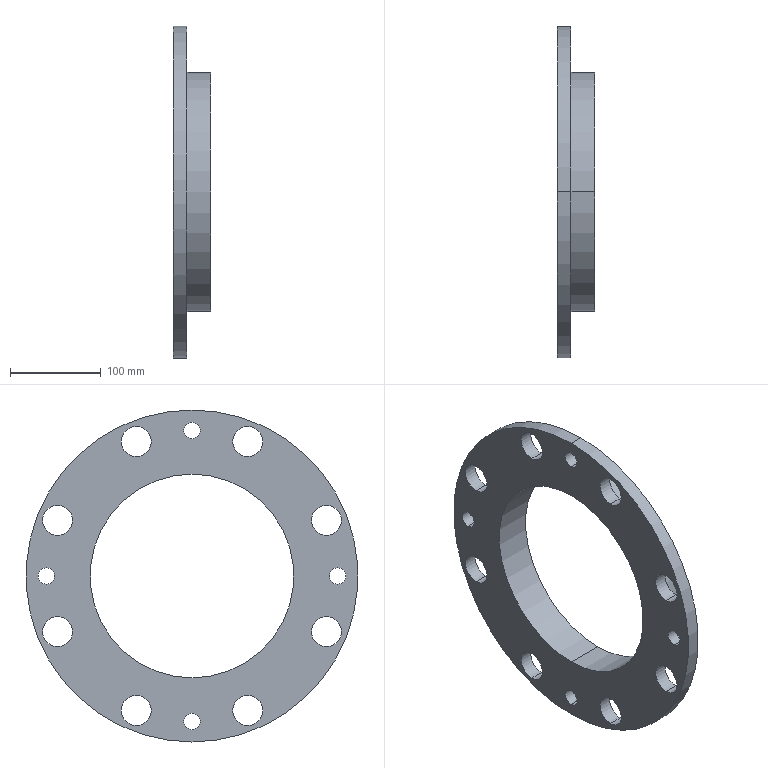Part | SolidWorks | features ICE 2, Revolution 1 | 1 solid | 33 faces | box 41 x 365 x 365 mm | volume 1248338 mm3 | cylinder 30 | plane 3 | commonest cylinder face diameters 33 x16 18 x8 224 x2 263 x2 365 x2
STEP:
#1=CARTESIAN_POINT('',(-4.589,0.,-169.));
#2=VERTEX_POINT('',#1);
#3=CARTESIAN_POINT('',(-4.589,0.,-151.));
#4=VERTEX_POINT('',#3);
#5=CARTESIAN_POINT('',(-4.589,0.,-160.));
#6=DIRECTION('',(-1.,0.,0.));
#7=DIRECTION('',(0.,0.,1.));
#8=AXIS2_PLACEMENT_3D('',#5,#6,#7);
#9=CIRCLE('',#8,9.);
#10=EDGE_CURVE('',#2,#4,#9,.T.);
#11=ORIENTED_EDGE('',*,*,#10,.F.);
#12=CARTESIAN_POINT('',(-19.589,0.,-169.));
#13=VERTEX_POINT('',#12);
#14=CARTESIAN_POINT('',(0.411,0.,-169.));
#15=DIRECTION('',(-1.,0.,0.));
#16=VECTOR('',#15,1000.);
#17=LINE('',#14,#16);
#18=EDGE_CURVE('',#2,#13,#17,.T.);
#19=ORIENTED_EDGE('',*,*,#18,.T.);
#20=CARTESIAN_POINT('',(-19.589,0.,-151.));
#21=VERTEX_POINT('',#20);
#22=CARTESIAN_POINT('',(-19.589,0.,-160.));
#23=DIRECTION('',(-1.,0.,0.));
#24=DIRECTION('',(0.,0.,1.));
#25=AXIS2_PLACEMENT_3D('',#22,#23,#24);
#26=CIRCLE('',#25,9.);
#27=EDGE_CURVE('',#13,#21,#26,.T.);
#28=ORIENTED_EDGE('',*,*,#27,.T.);
#29=CARTESIAN_POINT('',(0.411,0.,-151.));
#30=DIRECTION('',(-1.,0.,0.));
#31=VECTOR('',#30,1000.);
#32=LINE('',#29,#31);
#33=EDGE_CURVE('',#4,#21,#32,.T.);
#34=ORIENTED_EDGE('',*,*,#33,.F.);
#35=EDGE_LOOP('',(#11,#19,#28,#34));
#36=FACE_OUTER_BOUND('',#35,.T.);
#37=CARTESIAN_POINT('',(0.411,0.,-160.));
#38=DIRECTION('',(-1.,0.,0.));
#39=DIRECTION('',(0.,0.,1.));
#40=AXIS2_PLACEMENT_3D('',#37,#38,#39);
#41=CYLINDRICAL_SURFACE('',#40,9.);
#42=ADVANCED_FACE('',(#36),#41,.F.);
#43=CARTESIAN_POINT('',(-4.589,-160.,-9.));
#44=VERTEX_POINT('',#43);
#45=CARTESIAN_POINT('',(-4.589,-160.,9.));
#46=VERTEX_POINT('',#45);
#47=CARTESIAN_POINT('',(-4.589,-160.,0.));
#48=DIRECTION('',(-1.,0.,0.));
#49=DIRECTION('',(0.,0.,1.));
#50=AXIS2_PLACEMENT_3D('',#47,#48,#49);
#51=CIRCLE('',#50,9.);
#52=EDGE_CURVE('',#44,#46,#51,.T.);
#53=ORIENTED_EDGE('',*,*,#52,.F.);
#54=CARTESIAN_POINT('',(-19.589,-160.,-9.));
#55=VERTEX_POINT('',#54);
#56=CARTESIAN_POINT('',(0.411,-160.,-9.));
#57=DIRECTION('',(-1.,0.,0.));
#58=VECTOR('',#57,1000.);
#59=LINE('',#56,#58);
#60=EDGE_CURVE('',#44,#55,#59,.T.);
#61=ORIENTED_EDGE('',*,*,#60,.T.);
#62=CARTESIAN_POINT('',(-19.589,-160.,9.));
#63=VERTEX_POINT('',#62);
#64=CARTESIAN_POINT('',(-19.589,-160.,0.));
#65=DIRECTION('',(-1.,0.,0.));
#66=DIRECTION('',(0.,0.,1.));
#67=AXIS2_PLACEMENT_3D('',#64,#65,#66);
#68=CIRCLE('',#67,9.);
#69=EDGE_CURVE('',#55,#63,#68,.T.);
#70=ORIENTED_EDGE('',*,*,#69,.T.);
#71=CARTESIAN_POINT('',(0.411,-160.,9.));
#72=DIRECTION('',(-1.,0.,0.));
#73=VECTOR('',#72,1000.);
#74=LINE('',#71,#73);
#75=EDGE_CURVE('',#46,#63,#74,.T.);
#76=ORIENTED_EDGE('',*,*,#75,.F.);
#77=EDGE_LOOP('',(#53,#61,#70,#76));
#78=FACE_OUTER_BOUND('',#77,.T.);
#79=CARTESIAN_POINT('',(0.411,-160.,0.));
#80=DIRECTION('',(-1.,0.,0.));
#81=DIRECTION('',(0.,0.,1.));
#82=AXIS2_PLACEMENT_3D('',#79,#80,#81);
#83=CYLINDRICAL_SURFACE('',#82,9.);
#84=ADVANCED_FACE('',(#78),#83,.F.);
#85=CARTESIAN_POINT('',(-4.589,0.,151.));
#86=VERTEX_POINT('',#85);
#87=CARTESIAN_POINT('',(-4.589,0.,169.));
#88=VERTEX_POINT('',#87);
#89=CARTESIAN_POINT('',(-4.589,0.,160.));
#90=DIRECTION('',(-1.,0.,0.));
#91=DIRECTION('',(0.,0.,1.));
#92=AXIS2_PLACEMENT_3D('',#89,#90,#91);
#93=CIRCLE('',#92,9.);
#94=EDGE_CURVE('',#86,#88,#93,.T.);
#95=ORIENTED_EDGE('',*,*,#94,.F.);
#96=CARTESIAN_POINT('',(-19.589,0.,151.));
#97=VERTEX_POINT('',#96);
#98=CARTESIAN_POINT('',(0.411,0.,151.));
#99=DIRECTION('',(-1.,0.,0.));
#100=VECTOR('',#99,1000.);
#101=LINE('',#98,#100);
#102=EDGE_CURVE('',#86,#97,#101,.T.);
#103=ORIENTED_EDGE('',*,*,#102,.T.);
#104=CARTESIAN_POINT('',(-19.589,0.,169.));
#105=VERTEX_POINT('',#104);
#106=CARTESIAN_POINT('',(-19.589,0.,160.));
#107=DIRECTION('',(-1.,0.,0.));
#108=DIRECTION('',(0.,0.,1.));
#109=AXIS2_PLACEMENT_3D('',#106,#107,#108);
#110=CIRCLE('',#109,9.);
#111=EDGE_CURVE('',#97,#105,#110,.T.);
#112=ORIENTED_EDGE('',*,*,#111,.T.);
#113=CARTESIAN_POINT('',(0.411,0.,169.));
#114=DIRECTION('',(-1.,0.,0.));
#115=VECTOR('',#114,1000.);
#116=LINE('',#113,#115);
#117=EDGE_CURVE('',#88,#105,#116,.T.);
#118=ORIENTED_EDGE('',*,*,#117,.F.);
#119=EDGE_LOOP('',(#95,#103,#112,#118));
#120=FACE_OUTER_BOUND('',#119,.T.);
#121=CARTESIAN_POINT('',(0.411,0.,160.));
#122=DIRECTION('',(-1.,0.,0.));
#123=DIRECTION('',(0.,0.,1.));
#124=AXIS2_PLACEMENT_3D('',#121,#122,#123);
#125=CYLINDRICAL_SURFACE('',#124,9.);
#126=ADVANCED_FACE('',(#120),#125,.F.);
#127=CARTESIAN_POINT('',(-4.589,160.,-9.));
#128=VERTEX_POINT('',#127);
#129=CARTESIAN_POINT('',(-4.589,160.,9.));
#130=VERTEX_POINT('',#129);
#131=CARTESIAN_POINT('',(-4.589,160.,0.));
#132=DIRECTION('',(-1.,0.,0.));
#133=DIRECTION('',(0.,0.,1.));
#134=AXIS2_PLACEMENT_3D('',#131,#132,#133);
#135=CIRCLE('',#134,9.);
#136=EDGE_CURVE('',#128,#130,#135,.T.);
#137=ORIENTED_EDGE('',*,*,#136,.F.);
#138=CARTESIAN_POINT('',(-19.589,160.,-9.));
#139=VERTEX_POINT('',#138);
#140=CARTESIAN_POINT('',(0.411,160.,-9.));
#141=DIRECTION('',(-1.,0.,0.));
#142=VECTOR('',#141,1000.);
#143=LINE('',#140,#142);
#144=EDGE_CURVE('',#128,#139,#143,.T.);
#145=ORIENTED_EDGE('',*,*,#144,.T.);
#146=CARTESIAN_POINT('',(-19.589,160.,9.));
#147=VERTEX_POINT('',#146);
#148=CARTESIAN_POINT('',(-19.589,160.,0.));
#149=DIRECTION('',(-1.,0.,0.));
#150=DIRECTION('',(0.,0.,1.));
#151=AXIS2_PLACEMENT_3D('',#148,#149,#150);
#152=CIRCLE('',#151,9.);
#153=EDGE_CURVE('',#139,#147,#152,.T.);
#154=ORIENTED_EDGE('',*,*,#153,.T.);
#155=CARTESIAN_POINT('',(0.411,160.,9.));
#156=DIRECTION('',(-1.,0.,0.));
#157=VECTOR('',#156,1000.);
#158=LINE('',#155,#157);
#159=EDGE_CURVE('',#130,#147,#158,.T.);
#160=ORIENTED_EDGE('',*,*,#159,.F.);
#161=EDGE_LOOP('',(#137,#145,#154,#160));
#162=FACE_OUTER_BOUND('',#161,.T.);
#163=CARTESIAN_POINT('',(0.411,160.,0.));
#164=DIRECTION('',(-1.,0.,0.));
#165=DIRECTION('',(0.,0.,1.));
#166=AXIS2_PLACEMENT_3D('',#163,#164,#165);
#167=CYLINDRICAL_SURFACE('',#166,9.);
#168=ADVANCED_FACE('',(#162),#167,.F.);
#169=CARTESIAN_POINT('',(-4.589,147.821,-77.729));
#170=VERTEX_POINT('',#169);
#171=CARTESIAN_POINT('',(-4.589,147.821,-44.729));
#172=VERTEX_POINT('',#171);
#173=CARTESIAN_POINT('',(-4.589,147.821,-61.229));
#174=DIRECTION('',(-1.,0.,0.));
#175=DIRECTION('',(0.,0.,1.));
#176=AXIS2_PLACEMENT_3D('',#173,#174,#175);
#177=CIRCLE('',#176,16.5);
#178=EDGE_CURVE('',#170,#172,#177,.T.);
#179=ORIENTED_EDGE('',*,*,#178,.F.);
#180=CARTESIAN_POINT('',(-19.589,147.821,-77.729));
#181=VERTEX_POINT('',#180);
#182=CARTESIAN_POINT('',(0.411,147.821,-77.729));
#183=DIRECTION('',(-1.,0.,0.));
#184=VECTOR('',#183,1000.);
#185=LINE('',#182,#184);
#186=EDGE_CURVE('',#170,#181,#185,.T.);
#187=ORIENTED_EDGE('',*,*,#186,.T.);
#188=CARTESIAN_POINT('',(-19.589,147.821,-44.729));
#189=VERTEX_POINT('',#188);
#190=CARTESIAN_POINT('',(-19.589,147.821,-61.229));
#191=DIRECTION('',(-1.,0.,0.));
#192=DIRECTION('',(0.,0.,1.));
#193=AXIS2_PLACEMENT_3D('',#190,#191,#192);
#194=CIRCLE('',#193,16.5);
#195=EDGE_CURVE('',#181,#189,#194,.T.);
#196=ORIENTED_EDGE('',*,*,#195,.T.);
#197=CARTESIAN_POINT('',(0.411,147.821,-44.729));
#198=DIRECTION('',(-1.,0.,0.));
#199=VECTOR('',#198,1000.);
#200=LINE('',#197,#199);
#201=EDGE_CURVE('',#172,#189,#200,.T.);
#202=ORIENTED_EDGE('',*,*,#201,.F.);
#203=EDGE_LOOP('',(#179,#187,#196,#202));
#204=FACE_OUTER_BOUND('',#203,.T.);
#205=CARTESIAN_POINT('',(0.411,147.821,-61.229));
#206=DIRECTION('',(-1.,0.,0.));
#207=DIRECTION('',(0.,0.,1.));
#208=AXIS2_PLACEMENT_3D('',#205,#206,#207);
#209=CYLINDRICAL_SURFACE('',#208,16.5);
#210=ADVANCED_FACE('',(#204),#209,.F.);
#211=CARTESIAN_POINT('',(-4.589,61.229,-164.321));
#212=VERTEX_POINT('',#211);
#213=CARTESIAN_POINT('',(-4.589,61.229,-131.321));
#214=VERTEX_POINT('',#213);
#215=CARTESIAN_POINT('',(-4.589,61.229,-147.821));
#216=DIRECTION('',(-1.,0.,0.));
#217=DIRECTION('',(0.,0.,1.));
#218=AXIS2_PLACEMENT_3D('',#215,#216,#217);
#219=CIRCLE('',#218,16.5);
#220=EDGE_CURVE('',#212,#214,#219,.T.);
#221=ORIENTED_EDGE('',*,*,#220,.F.);
#222=CARTESIAN_POINT('',(-19.589,61.229,-164.321));
#223=VERTEX_POINT('',#222);
#224=CARTESIAN_POINT('',(0.411,61.229,-164.321));
#225=DIRECTION('',(-1.,0.,0.));
#226=VECTOR('',#225,1000.);
#227=LINE('',#224,#226);
#228=EDGE_CURVE('',#212,#223,#227,.T.);
#229=ORIENTED_EDGE('',*,*,#228,.T.);
#230=CARTESIAN_POINT('',(-19.589,61.229,-131.321));
#231=VERTEX_POINT('',#230);
#232=CARTESIAN_POINT('',(-19.589,61.229,-147.821));
#233=DIRECTION('',(-1.,0.,0.));
#234=DIRECTION('',(0.,0.,1.));
#235=AXIS2_PLACEMENT_3D('',#232,#233,#234);
#236=CIRCLE('',#235,16.5);
#237=EDGE_CURVE('',#223,#231,#236,.T.);
#238=ORIENTED_EDGE('',*,*,#237,.T.);
#239=CARTESIAN_POINT('',(0.411,61.229,-131.321));
#240=DIRECTION('',(-1.,0.,0.));
#241=VECTOR('',#240,1000.);
#242=LINE('',#239,#241);
#243=EDGE_CURVE('',#214,#231,#242,.T.);
#244=ORIENTED_EDGE('',*,*,#243,.F.);
#245=EDGE_LOOP('',(#221,#229,#238,#244));
#246=FACE_OUTER_BOUND('',#245,.T.);
#247=CARTESIAN_POINT('',(0.411,61.229,-147.821));
#248=DIRECTION('',(-1.,0.,0.));
#249=DIRECTION('',(0.,0.,1.));
#250=AXIS2_PLACEMENT_3D('',#247,#248,#249);
#251=CYLINDRICAL_SURFACE('',#250,16.5);
#252=ADVANCED_FACE('',(#246),#251,.F.);
#253=CARTESIAN_POINT('',(-4.589,-61.229,-164.321));
#254=VERTEX_POINT('',#253);
#255=CARTESIAN_POINT('',(-4.589,-61.229,-131.321));
#256=VERTEX_POINT('',#255);
#257=CARTESIAN_POINT('',(-4.589,-61.229,-147.821));
#258=DIRECTION('',(-1.,0.,0.));
#259=DIRECTION('',(0.,0.,1.));
#260=AXIS2_PLACEMENT_3D('',#257,#258,#259);
#261=CIRCLE('',#260,16.5);
#262=EDGE_CURVE('',#254,#256,#261,.T.);
#263=ORIENTED_EDGE('',*,*,#262,.F.);
#264=CARTESIAN_POINT('',(-19.589,-61.229,-164.321));
#265=VERTEX_POINT('',#264);
#266=CARTESIAN_POINT('',(0.411,-61.229,-164.321));
#267=DIRECTION('',(-1.,0.,0.));
#268=VECTOR('',#267,1000.);
#269=LINE('',#266,#268);
#270=EDGE_CURVE('',#254,#265,#269,.T.);
#271=ORIENTED_EDGE('',*,*,#270,.T.);
#272=CARTESIAN_POINT('',(-19.589,-61.229,-131.321));
#273=VERTEX_POINT('',#272);
#274=CARTESIAN_POINT('',(-19.589,-61.229,-147.821));
#275=DIRECTION('',(-1.,0.,0.));
#276=DIRECTION('',(0.,0.,1.));
#277=AXIS2_PLACEMENT_3D('',#274,#275,#276);
#278=CIRCLE('',#277,16.5);
#279=EDGE_CURVE('',#265,#273,#278,.T.);
#280=ORIENTED_EDGE('',*,*,#279,.T.);
#281=CARTESIAN_POINT('',(0.411,-61.229,-131.321));
#282=DIRECTION('',(-1.,0.,0.));
#283=VECTOR('',#282,1000.);
#284=LINE('',#281,#283);
#285=EDGE_CURVE('',#256,#273,#284,.T.);
#286=ORIENTED_EDGE('',*,*,#285,.F.);
#287=EDGE_LOOP('',(#263,#271,#280,#286));
#288=FACE_OUTER_BOUND('',#287,.T.);
#289=CARTESIAN_POINT('',(0.411,-61.229,-147.821));
#290=DIRECTION('',(-1.,0.,0.));
#291=DIRECTION('',(0.,0.,1.));
#292=AXIS2_PLACEMENT_3D('',#289,#290,#291);
#293=CYLINDRICAL_SURFACE('',#292,16.5);
#294=ADVANCED_FACE('',(#288),#293,.F.);
#295=CARTESIAN_POINT('',(-4.589,-147.821,-77.729));
#296=VERTEX_POINT('',#295);
#297=CARTESIAN_POINT('',(-4.589,-147.821,-44.729));
#298=VERTEX_POINT('',#297);
#299=CARTESIAN_POINT('',(-4.589,-147.821,-61.229));
#300=DIRECTION('',(-1.,0.,0.));
#301=DIRECTION('',(0.,0.,1.));
#302=AXIS2_PLACEMENT_3D('',#299,#300,#301);
#303=CIRCLE('',#302,16.5);
#304=EDGE_CURVE('',#296,#298,#303,.T.);
#305=ORIENTED_EDGE('',*,*,#304,.F.);
#306=CARTESIAN_POINT('',(-19.589,-147.821,-77.729));
#307=VERTEX_POINT('',#306);
#308=CARTESIAN_POINT('',(0.411,-147.821,-77.729));
#309=DIRECTION('',(-1.,0.,0.));
#310=VECTOR('',#309,1000.);
#311=LINE('',#308,#310);
#312=EDGE_CURVE('',#296,#307,#311,.T.);
#313=ORIENTED_EDGE('',*,*,#312,.T.);
#314=CARTESIAN_POINT('',(-19.589,-147.821,-44.729));
#315=VERTEX_POINT('',#314);
#316=CARTESIAN_POINT('',(-19.589,-147.821,-61.229));
#317=DIRECTION('',(-1.,0.,0.));
#318=DIRECTION('',(0.,0.,1.));
#319=AXIS2_PLACEMENT_3D('',#316,#317,#318);
#320=CIRCLE('',#319,16.5);
#321=EDGE_CURVE('',#307,#315,#320,.T.);
#322=ORIENTED_EDGE('',*,*,#321,.T.);
#323=CARTESIAN_POINT('',(0.411,-147.821,-44.729));
#324=DIRECTION('',(-1.,0.,0.));
#325=VECTOR('',#324,1000.);
#326=LINE('',#323,#325);
#327=EDGE_CURVE('',#298,#315,#326,.T.);
#328=ORIENTED_EDGE('',*,*,#327,.F.);
#329=EDGE_LOOP('',(#305,#313,#322,#328));
#330=FACE_OUTER_BOUND('',#329,.T.);
#331=CARTESIAN_POINT('',(0.411,-147.821,-61.229));
#332=DIRECTION('',(-1.,0.,0.));
#333=DIRECTION('',(0.,0.,1.));
#334=AXIS2_PLACEMENT_3D('',#331,#332,#333);
#335=CYLINDRICAL_SURFACE('',#334,16.5);
#336=ADVANCED_FACE('',(#330),#335,.F.);
#337=CARTESIAN_POINT('',(-4.589,-147.821,44.729));
#338=VERTEX_POINT('',#337);
#339=CARTESIAN_POINT('',(-4.589,-147.821,77.729));
#340=VERTEX_POINT('',#339);
#341=CARTESIAN_POINT('',(-4.589,-147.821,61.229));
#342=DIRECTION('',(-1.,0.,0.));
#343=DIRECTION('',(0.,0.,1.));
#344=AXIS2_PLACEMENT_3D('',#341,#342,#343);
#345=CIRCLE('',#344,16.5);
#346=EDGE_CURVE('',#338,#340,#345,.T.);
#347=ORIENTED_EDGE('',*,*,#346,.F.);
#348=CARTESIAN_POINT('',(-19.589,-147.821,44.729));
#349=VERTEX_POINT('',#348);
#350=CARTESIAN_POINT('',(0.411,-147.821,44.729));
#351=DIRECTION('',(-1.,0.,0.));
#352=VECTOR('',#351,1000.);
#353=LINE('',#350,#352);
#354=EDGE_CURVE('',#338,#349,#353,.T.);
#355=ORIENTED_EDGE('',*,*,#354,.T.);
#356=CARTESIAN_POINT('',(-19.589,-147.821,77.729));
#357=VERTEX_POINT('',#356);
#358=CARTESIAN_POINT('',(-19.589,-147.821,61.229));
#359=DIRECTION('',(-1.,0.,0.));
#360=DIRECTION('',(0.,0.,1.));
#361=AXIS2_PLACEMENT_3D('',#358,#359,#360);
#362=CIRCLE('',#361,16.5);
#363=EDGE_CURVE('',#349,#357,#362,.T.);
#364=ORIENTED_EDGE('',*,*,#363,.T.);
#365=CARTESIAN_POINT('',(0.411,-147.821,77.729));
#366=DIRECTION('',(-1.,0.,0.));
#367=VECTOR('',#366,1000.);
#368=LINE('',#365,#367);
#369=EDGE_CURVE('',#340,#357,#368,.T.);
#370=ORIENTED_EDGE('',*,*,#369,.F.);
#371=EDGE_LOOP('',(#347,#355,#364,#370));
#372=FACE_OUTER_BOUND('',#371,.T.);
#373=CARTESIAN_POINT('',(0.411,-147.821,61.229));
#374=DIRECTION('',(-1.,0.,0.));
#375=DIRECTION('',(0.,0.,1.));
#376=AXIS2_PLACEMENT_3D('',#373,#374,#375);
#377=CYLINDRICAL_SURFACE('',#376,16.5);
#378=ADVANCED_FACE('',(#372),#377,.F.);
#379=CARTESIAN_POINT('',(-4.589,-61.229,131.321));
#380=VERTEX_POINT('',#379);
#381=CARTESIAN_POINT('',(-4.589,-61.229,164.321));
#382=VERTEX_POINT('',#381);
#383=CARTESIAN_POINT('',(-4.589,-61.229,147.821));
#384=DIRECTION('',(-1.,0.,0.));
#385=DIRECTION('',(0.,0.,1.));
#386=AXIS2_PLACEMENT_3D('',#383,#384,#385);
#387=CIRCLE('',#386,16.5);
#388=EDGE_CURVE('',#380,#382,#387,.T.);
#389=ORIENTED_EDGE('',*,*,#388,.F.);
#390=CARTESIAN_POINT('',(-19.589,-61.229,131.321));
#391=VERTEX_POINT('',#390);
#392=CARTESIAN_POINT('',(0.411,-61.229,131.321));
#393=DIRECTION('',(-1.,0.,0.));
#394=VECTOR('',#393,1000.);
#395=LINE('',#392,#394);
#396=EDGE_CURVE('',#380,#391,#395,.T.);
#397=ORIENTED_EDGE('',*,*,#396,.T.);
#398=CARTESIAN_POINT('',(-19.589,-61.229,164.321));
#399=VERTEX_POINT('',#398);
#400=CARTESIAN_POINT('',(-19.589,-61.229,147.821));
#401=DIRECTION('',(-1.,0.,0.));
#402=DIRECTION('',(0.,0.,1.));
#403=AXIS2_PLACEMENT_3D('',#400,#401,#402);
#404=CIRCLE('',#403,16.5);
#405=EDGE_CURVE('',#391,#399,#404,.T.);
#406=ORIENTED_EDGE('',*,*,#405,.T.);
#407=CARTESIAN_POINT('',(0.411,-61.229,164.321));
#408=DIRECTION('',(-1.,0.,0.));
#409=VECTOR('',#408,1000.);
#410=LINE('',#407,#409);
#411=EDGE_CURVE('',#382,#399,#410,.T.);
#412=ORIENTED_EDGE('',*,*,#411,.F.);
#413=EDGE_LOOP('',(#389,#397,#406,#412));
#414=FACE_OUTER_BOUND('',#413,.T.);
#415=CARTESIAN_POINT('',(0.411,-61.229,147.821));
#416=DIRECTION('',(-1.,0.,0.));
#417=DIRECTION('',(0.,0.,1.));
#418=AXIS2_PLACEMENT_3D('',#415,#416,#417);
#419=CYLINDRICAL_SURFACE('',#418,16.5);
#420=ADVANCED_FACE('',(#414),#419,.F.);
#421=CARTESIAN_POINT('',(-4.589,61.229,131.321));
#422=VERTEX_POINT('',#421);
#423=CARTESIAN_POINT('',(-4.589,61.229,164.321));
#424=VERTEX_POINT('',#423);
#425=CARTESIAN_POINT('',(-4.589,61.229,147.821));
#426=DIRECTION('',(-1.,0.,0.));
#427=DIRECTION('',(0.,0.,1.));
#428=AXIS2_PLACEMENT_3D('',#425,#426,#427);
#429=CIRCLE('',#428,16.5);
#430=EDGE_CURVE('',#422,#424,#429,.T.);
#431=ORIENTED_EDGE('',*,*,#430,.F.);
#432=CARTESIAN_POINT('',(-19.589,61.229,131.321));
#433=VERTEX_POINT('',#432);
#434=CARTESIAN_POINT('',(0.411,61.229,131.321));
#435=DIRECTION('',(-1.,0.,0.));
#436=VECTOR('',#435,1000.);
#437=LINE('',#434,#436);
#438=EDGE_CURVE('',#422,#433,#437,.T.);
#439=ORIENTED_EDGE('',*,*,#438,.T.);
#440=CARTESIAN_POINT('',(-19.589,61.229,164.321));
#441=VERTEX_POINT('',#440);
#442=CARTESIAN_POINT('',(-19.589,61.229,147.821));
#443=DIRECTION('',(-1.,0.,0.));
#444=DIRECTION('',(0.,0.,1.));
#445=AXIS2_PLACEMENT_3D('',#442,#443,#444);
#446=CIRCLE('',#445,16.5);
#447=EDGE_CURVE('',#433,#441,#446,.T.);
#448=ORIENTED_EDGE('',*,*,#447,.T.);
#449=CARTESIAN_POINT('',(0.411,61.229,164.321));
#450=DIRECTION('',(-1.,0.,0.));
#451=VECTOR('',#450,1000.);
#452=LINE('',#449,#451);
#453=EDGE_CURVE('',#424,#441,#452,.T.);
#454=ORIENTED_EDGE('',*,*,#453,.F.);
#455=EDGE_LOOP('',(#431,#439,#448,#454));
#456=FACE_OUTER_BOUND('',#455,.T.);
#457=CARTESIAN_POINT('',(0.411,61.229,147.821));
#458=DIRECTION('',(-1.,0.,0.));
#459=DIRECTION('',(0.,0.,1.));
#460=AXIS2_PLACEMENT_3D('',#457,#458,#459);
#461=CYLINDRICAL_SURFACE('',#460,16.5);
#462=ADVANCED_FACE('',(#456),#461,.F.);
#463=CARTESIAN_POINT('',(-4.589,147.821,44.729));
#464=VERTEX_POINT('',#463);
#465=CARTESIAN_POINT('',(-4.589,147.821,77.729));
#466=VERTEX_POINT('',#465);
#467=CARTESIAN_POINT('',(-4.589,147.821,61.229));
#468=DIRECTION('',(-1.,0.,0.));
#469=DIRECTION('',(0.,0.,1.));
#470=AXIS2_PLACEMENT_3D('',#467,#468,#469);
#471=CIRCLE('',#470,16.5);
#472=EDGE_CURVE('',#464,#466,#471,.T.);
#473=ORIENTED_EDGE('',*,*,#472,.F.);
#474=CARTESIAN_POINT('',(-19.589,147.821,44.729));
#475=VERTEX_POINT('',#474);
#476=CARTESIAN_POINT('',(0.411,147.821,44.729));
#477=DIRECTION('',(-1.,0.,0.));
#478=VECTOR('',#477,1000.);
#479=LINE('',#476,#478);
#480=EDGE_CURVE('',#464,#475,#479,.T.);
#481=ORIENTED_EDGE('',*,*,#480,.T.);
#482=CARTESIAN_POINT('',(-19.589,147.821,77.729));
#483=VERTEX_POINT('',#482);
#484=CARTESIAN_POINT('',(-19.589,147.821,61.229));
#485=DIRECTION('',(-1.,0.,0.));
#486=DIRECTION('',(0.,0.,1.));
#487=AXIS2_PLACEMENT_3D('',#484,#485,#486);
#488=CIRCLE('',#487,16.5);
#489=EDGE_CURVE('',#475,#483,#488,.T.);
#490=ORIENTED_EDGE('',*,*,#489,.T.);
#491=CARTESIAN_POINT('',(0.411,147.821,77.729));
#492=DIRECTION('',(-1.,0.,0.));
#493=VECTOR('',#492,1000.);
#494=LINE('',#491,#493);
#495=EDGE_CURVE('',#466,#483,#494,.T.);
#496=ORIENTED_EDGE('',*,*,#495,.F.);
#497=EDGE_LOOP('',(#473,#481,#490,#496));
#498=FACE_OUTER_BOUND('',#497,.T.);
#499=CARTESIAN_POINT('',(0.411,147.821,61.229));
#500=DIRECTION('',(-1.,0.,0.));
#501=DIRECTION('',(0.,0.,1.));
#502=AXIS2_PLACEMENT_3D('',#499,#500,#501);
#503=CYLINDRICAL_SURFACE('',#502,16.5);
#504=ADVANCED_FACE('',(#498),#503,.F.);
#505=CARTESIAN_POINT('',(21.411,0.,131.5));
#506=VERTEX_POINT('',#505);
#507=CARTESIAN_POINT('',(21.411,0.,-131.5));
#508=VERTEX_POINT('',#507);
#509=CARTESIAN_POINT('',(21.411,0.,0.));
#510=DIRECTION('',(-1.,0.,0.));
#511=DIRECTION('',(0.,0.,1.));
#512=AXIS2_PLACEMENT_3D('',#509,#510,#511);
#513=CIRCLE('',#512,131.5);
#514=EDGE_CURVE('',#506,#508,#513,.T.);
#515=ORIENTED_EDGE('',*,*,#514,.T.);
#516=CARTESIAN_POINT('',(-4.589,0.,-131.5));
#517=VERTEX_POINT('',#516);
#518=CARTESIAN_POINT('',(-91.426,0.,-131.5));
#519=DIRECTION('',(-1.,0.,0.));
#520=VECTOR('',#519,1000.);
#521=LINE('',#518,#520);
#522=EDGE_CURVE('',#508,#517,#521,.T.);
#523=ORIENTED_EDGE('',*,*,#522,.T.);
#524=CARTESIAN_POINT('',(-4.589,0.,131.5));
#525=VERTEX_POINT('',#524);
#526=CARTESIAN_POINT('',(-4.589,0.,0.));
#527=DIRECTION('',(-1.,0.,0.));
#528=DIRECTION('',(0.,0.,1.));
#529=AXIS2_PLACEMENT_3D('',#526,#527,#528);
#530=CIRCLE('',#529,131.5);
#531=EDGE_CURVE('',#525,#517,#530,.T.);
#532=ORIENTED_EDGE('',*,*,#531,.F.);
#533=CARTESIAN_POINT('',(-91.426,0.,131.5));
#534=DIRECTION('',(-1.,0.,0.));
#535=VECTOR('',#534,1000.);
#536=LINE('',#533,#535);
#537=EDGE_CURVE('',#506,#525,#536,.T.);
#538=ORIENTED_EDGE('',*,*,#537,.F.);
#539=EDGE_LOOP('',(#515,#523,#532,#538));
#540=FACE_OUTER_BOUND('',#539,.T.);
#541=CARTESIAN_POINT('',(-91.426,0.,0.));
#542=DIRECTION('',(-1.,0.,0.));
#543=DIRECTION('',(0.,0.,1.));
#544=AXIS2_PLACEMENT_3D('',#541,#542,#543);
#545=CYLINDRICAL_SURFACE('',#544,131.5);
#546=ADVANCED_FACE('',(#540),#545,.T.);
#547=CARTESIAN_POINT('',(-4.589,0.,182.5));
#548=VERTEX_POINT('',#547);
#549=CARTESIAN_POINT('',(-4.589,0.,-182.5));
#550=VERTEX_POINT('',#549);
#551=CARTESIAN_POINT('',(-4.589,0.,0.));
#552=DIRECTION('',(-1.,0.,0.));
#553=DIRECTION('',(0.,0.,1.));
#554=AXIS2_PLACEMENT_3D('',#551,#552,#553);
#555=CIRCLE('',#554,182.5);
#556=EDGE_CURVE('',#548,#550,#555,.T.);
#557=ORIENTED_EDGE('',*,*,#556,.T.);
#558=CARTESIAN_POINT('',(-19.589,0.,-182.5));
#559=VERTEX_POINT('',#558);
#560=CARTESIAN_POINT('',(-91.426,0.,-182.5));
#561=DIRECTION('',(-1.,0.,0.));
#562=VECTOR('',#561,1000.);
#563=LINE('',#560,#562);
#564=EDGE_CURVE('',#550,#559,#563,.T.);
#565=ORIENTED_EDGE('',*,*,#564,.T.);
#566=CARTESIAN_POINT('',(-19.589,0.,182.5));
#567=VERTEX_POINT('',#566);
#568=CARTESIAN_POINT('',(-19.589,0.,0.));
#569=DIRECTION('',(-1.,0.,0.));
#570=DIRECTION('',(0.,0.,1.));
#571=AXIS2_PLACEMENT_3D('',#568,#569,#570);
#572=CIRCLE('',#571,182.5);
#573=EDGE_CURVE('',#567,#559,#572,.T.);
#574=ORIENTED_EDGE('',*,*,#573,.F.);
#575=CARTESIAN_POINT('',(-91.426,0.,182.5));
#576=DIRECTION('',(-1.,0.,0.));
#577=VECTOR('',#576,1000.);
#578=LINE('',#575,#577);
#579=EDGE_CURVE('',#548,#567,#578,.T.);
#580=ORIENTED_EDGE('',*,*,#579,.F.);
#581=EDGE_LOOP('',(#557,#565,#574,#580));
#582=FACE_OUTER_BOUND('',#581,.T.);
#583=CARTESIAN_POINT('',(-91.426,0.,0.));
#584=DIRECTION('',(-1.,0.,0.));
#585=DIRECTION('',(0.,0.,1.));
#586=AXIS2_PLACEMENT_3D('',#583,#584,#585);
#587=CYLINDRICAL_SURFACE('',#586,182.5);
#588=ADVANCED_FACE('',(#582),#587,.T.);
#589=CARTESIAN_POINT('',(21.411,0.,-112.));
#590=VERTEX_POINT('',#589);
#591=CARTESIAN_POINT('',(21.411,0.,112.));
#592=VERTEX_POINT('',#591);
#593=CARTESIAN_POINT('',(21.411,0.,0.));
#594=DIRECTION('',(-1.,0.,0.));
#595=DIRECTION('',(0.,0.,1.));
#596=AXIS2_PLACEMENT_3D('',#593,#594,#595);
#597=CIRCLE('',#596,112.);
#598=EDGE_CURVE('',#590,#592,#597,.T.);
#599=ORIENTED_EDGE('',*,*,#598,.F.);
#600=CARTESIAN_POINT('',(-19.589,0.,-112.));
#601=VERTEX_POINT('',#600);
#602=CARTESIAN_POINT('',(-91.426,0.,-112.));
#603=DIRECTION('',(-1.,0.,0.));
#604=VECTOR('',#603,1000.);
#605=LINE('',#602,#604);
#606=EDGE_CURVE('',#590,#601,#605,.T.);
#607=ORIENTED_EDGE('',*,*,#606,.T.);
#608=CARTESIAN_POINT('',(-19.589,0.,112.));
#609=VERTEX_POINT('',#608);
#610=CARTESIAN_POINT('',(-19.589,0.,0.));
#611=DIRECTION('',(-1.,0.,0.));
#612=DIRECTION('',(0.,0.,1.));
#613=AXIS2_PLACEMENT_3D('',#610,#611,#612);
#614=CIRCLE('',#613,112.);
#615=EDGE_CURVE('',#601,#609,#614,.T.);
#616=ORIENTED_EDGE('',*,*,#615,.T.);
#617=CARTESIAN_POINT('',(-91.426,0.,112.));
#618=DIRECTION('',(-1.,0.,0.));
#619=VECTOR('',#618,1000.);
#620=LINE('',#617,#619);
#621=EDGE_CURVE('',#592,#609,#620,.T.);
#622=ORIENTED_EDGE('',*,*,#621,.F.);
#623=EDGE_LOOP('',(#599,#607,#616,#622));
#624=FACE_OUTER_BOUND('',#623,.T.);
#625=CARTESIAN_POINT('',(-91.426,0.,0.));
#626=DIRECTION('',(-1.,0.,0.));
#627=DIRECTION('',(0.,0.,1.));
#628=AXIS2_PLACEMENT_3D('',#625,#626,#627);
#629=CYLINDRICAL_SURFACE('',#628,112.);
#630=ADVANCED_FACE('',(#624),#629,.F.);
#631=ORIENTED_EDGE('',*,*,#606,.F.);
#632=CARTESIAN_POINT('',(21.411,0.,0.));
#633=DIRECTION('',(-1.,0.,0.));
#634=DIRECTION('',(0.,0.,1.));
#635=AXIS2_PLACEMENT_3D('',#632,#633,#634);
#636=CIRCLE('',#635,112.);
#637=EDGE_CURVE('',#592,#590,#636,.T.);
#638=ORIENTED_EDGE('',*,*,#637,.F.);
#639=ORIENTED_EDGE('',*,*,#621,.T.);
#640=CARTESIAN_POINT('',(-19.589,0.,0.));
#641=DIRECTION('',(-1.,0.,0.));
#642=DIRECTION('',(0.,0.,1.));
#643=AXIS2_PLACEMENT_3D('',#640,#641,#642);
#644=CIRCLE('',#643,112.);
#645=EDGE_CURVE('',#609,#601,#644,.T.);
#646=ORIENTED_EDGE('',*,*,#645,.T.);
#647=EDGE_LOOP('',(#631,#638,#639,#646));
#648=FACE_OUTER_BOUND('',#647,.T.);
#649=CARTESIAN_POINT('',(-91.426,0.,0.));
#650=DIRECTION('',(-1.,0.,0.));
#651=DIRECTION('',(0.,0.,1.));
#652=AXIS2_PLACEMENT_3D('',#649,#650,#651);
#653=CYLINDRICAL_SURFACE('',#652,112.);
#654=ADVANCED_FACE('',(#648),#653,.F.);
#655=CARTESIAN_POINT('',(-19.589,0.,-160.));
#656=DIRECTION('',(-1.,0.,0.));
#657=DIRECTION('',(0.,0.,1.));
#658=AXIS2_PLACEMENT_3D('',#655,#656,#657);
#659=CIRCLE('',#658,9.);
#660=EDGE_CURVE('',#21,#13,#659,.T.);
#661=ORIENTED_EDGE('',*,*,#660,.F.);
#662=ORIENTED_EDGE('',*,*,#27,.F.);
#663=EDGE_LOOP('',(#661,#662));
#664=FACE_BOUND('',#663,.T.);
#665=CARTESIAN_POINT('',(-19.589,-160.,0.));
#666=DIRECTION('',(-1.,0.,0.));
#667=DIRECTION('',(0.,0.,1.));
#668=AXIS2_PLACEMENT_3D('',#665,#666,#667);
#669=CIRCLE('',#668,9.);
#670=EDGE_CURVE('',#63,#55,#669,.T.);
#671=ORIENTED_EDGE('',*,*,#670,.F.);
#672=ORIENTED_EDGE('',*,*,#69,.F.);
#673=EDGE_LOOP('',(#671,#672));
#674=FACE_BOUND('',#673,.T.);
#675=CARTESIAN_POINT('',(-19.589,0.,160.));
#676=DIRECTION('',(-1.,0.,0.));
#677=DIRECTION('',(0.,0.,1.));
#678=AXIS2_PLACEMENT_3D('',#675,#676,#677);
#679=CIRCLE('',#678,9.);
#680=EDGE_CURVE('',#105,#97,#679,.T.);
#681=ORIENTED_EDGE('',*,*,#680,.F.);
#682=ORIENTED_EDGE('',*,*,#111,.F.);
#683=EDGE_LOOP('',(#681,#682));
#684=FACE_BOUND('',#683,.T.);
#685=CARTESIAN_POINT('',(-19.589,160.,0.));
#686=DIRECTION('',(-1.,0.,0.));
#687=DIRECTION('',(0.,0.,1.));
#688=AXIS2_PLACEMENT_3D('',#685,#686,#687);
#689=CIRCLE('',#688,9.);
#690=EDGE_CURVE('',#147,#139,#689,.T.);
#691=ORIENTED_EDGE('',*,*,#690,.F.);
#692=ORIENTED_EDGE('',*,*,#153,.F.);
#693=EDGE_LOOP('',(#691,#692));
#694=FACE_BOUND('',#693,.T.);
#695=CARTESIAN_POINT('',(-19.589,147.821,-61.229));
#696=DIRECTION('',(-1.,0.,0.));
#697=DIRECTION('',(0.,0.,1.));
#698=AXIS2_PLACEMENT_3D('',#695,#696,#697);
#699=CIRCLE('',#698,16.5);
#700=EDGE_CURVE('',#189,#181,#699,.T.);
#701=ORIENTED_EDGE('',*,*,#700,.F.);
#702=ORIENTED_EDGE('',*,*,#195,.F.);
#703=EDGE_LOOP('',(#701,#702));
#704=FACE_BOUND('',#703,.T.);
#705=CARTESIAN_POINT('',(-19.589,61.229,-147.821));
#706=DIRECTION('',(-1.,0.,0.));
#707=DIRECTION('',(0.,0.,1.));
#708=AXIS2_PLACEMENT_3D('',#705,#706,#707);
#709=CIRCLE('',#708,16.5);
#710=EDGE_CURVE('',#231,#223,#709,.T.);
#711=ORIENTED_EDGE('',*,*,#710,.F.);
#712=ORIENTED_EDGE('',*,*,#237,.F.);
#713=EDGE_LOOP('',(#711,#712));
#714=FACE_BOUND('',#713,.T.);
#715=CARTESIAN_POINT('',(-19.589,-61.229,-147.821));
#716=DIRECTION('',(-1.,0.,0.));
#717=DIRECTION('',(0.,0.,1.));
#718=AXIS2_PLACEMENT_3D('',#715,#716,#717);
#719=CIRCLE('',#718,16.5);
#720=EDGE_CURVE('',#273,#265,#719,.T.);
#721=ORIENTED_EDGE('',*,*,#720,.F.);
#722=ORIENTED_EDGE('',*,*,#279,.F.);
#723=EDGE_LOOP('',(#721,#722));
#724=FACE_BOUND('',#723,.T.);
#725=CARTESIAN_POINT('',(-19.589,-147.821,-61.229));
#726=DIRECTION('',(-1.,0.,0.));
#727=DIRECTION('',(0.,0.,1.));
#728=AXIS2_PLACEMENT_3D('',#725,#726,#727);
#729=CIRCLE('',#728,16.5);
#730=EDGE_CURVE('',#315,#307,#729,.T.);
#731=ORIENTED_EDGE('',*,*,#730,.F.);
#732=ORIENTED_EDGE('',*,*,#321,.F.);
#733=EDGE_LOOP('',(#731,#732));
#734=FACE_BOUND('',#733,.T.);
#735=CARTESIAN_POINT('',(-19.589,-147.821,61.229));
#736=DIRECTION('',(-1.,0.,0.));
#737=DIRECTION('',(0.,0.,1.));
#738=AXIS2_PLACEMENT_3D('',#735,#736,#737);
#739=CIRCLE('',#738,16.5);
#740=EDGE_CURVE('',#357,#349,#739,.T.);
#741=ORIENTED_EDGE('',*,*,#740,.F.);
#742=ORIENTED_EDGE('',*,*,#363,.F.);
#743=EDGE_LOOP('',(#741,#742));
#744=FACE_BOUND('',#743,.T.);
#745=CARTESIAN_POINT('',(-19.589,-61.229,147.821));
#746=DIRECTION('',(-1.,0.,0.));
#747=DIRECTION('',(0.,0.,1.));
#748=AXIS2_PLACEMENT_3D('',#745,#746,#747);
#749=CIRCLE('',#748,16.5);
#750=EDGE_CURVE('',#399,#391,#749,.T.);
#751=ORIENTED_EDGE('',*,*,#750,.F.);
#752=ORIENTED_EDGE('',*,*,#405,.F.);
#753=EDGE_LOOP('',(#751,#752));
#754=FACE_BOUND('',#753,.T.);
#755=CARTESIAN_POINT('',(-19.589,61.229,147.821));
#756=DIRECTION('',(-1.,0.,0.));
#757=DIRECTION('',(0.,0.,1.));
#758=AXIS2_PLACEMENT_3D('',#755,#756,#757);
#759=CIRCLE('',#758,16.5);
#760=EDGE_CURVE('',#441,#433,#759,.T.);
#761=ORIENTED_EDGE('',*,*,#760,.F.);
#762=ORIENTED_EDGE('',*,*,#447,.F.);
#763=EDGE_LOOP('',(#761,#762));
#764=FACE_BOUND('',#763,.T.);
#765=CARTESIAN_POINT('',(-19.589,147.821,61.229));
#766=DIRECTION('',(-1.,0.,0.));
#767=DIRECTION('',(0.,0.,1.));
#768=AXIS2_PLACEMENT_3D('',#765,#766,#767);
#769=CIRCLE('',#768,16.5);
#770=EDGE_CURVE('',#483,#475,#769,.T.);
#771=ORIENTED_EDGE('',*,*,#770,.F.);
#772=ORIENTED_EDGE('',*,*,#489,.F.);
#773=EDGE_LOOP('',(#771,#772));
#774=FACE_BOUND('',#773,.T.);
#775=ORIENTED_EDGE('',*,*,#645,.F.);
#776=ORIENTED_EDGE('',*,*,#615,.F.);
#777=EDGE_LOOP('',(#775,#776));
#778=FACE_BOUND('',#777,.T.);
#779=ORIENTED_EDGE('',*,*,#573,.T.);
#780=CARTESIAN_POINT('',(-19.589,0.,0.));
#781=DIRECTION('',(-1.,0.,0.));
#782=DIRECTION('',(0.,0.,1.));
#783=AXIS2_PLACEMENT_3D('',#780,#781,#782);
#784=CIRCLE('',#783,182.5);
#785=EDGE_CURVE('',#559,#567,#784,.T.);
#786=ORIENTED_EDGE('',*,*,#785,.T.);
#787=EDGE_LOOP('',(#779,#786));
#788=FACE_OUTER_BOUND('',#787,.T.);
#789=CARTESIAN_POINT('',(-19.589,112.,0.));
#790=DIRECTION('',(1.,0.,0.));
#791=DIRECTION('',(0.,0.,-1.));
#792=AXIS2_PLACEMENT_3D('',#789,#790,#791);
#793=PLANE('',#792);
#794=ADVANCED_FACE('',(#664,#674,#684,#694,#704,#714,#724,#734,#744,#754,#764,#774,#778,#788),#793,.F.);
#795=ORIENTED_EDGE('',*,*,#564,.F.);
#796=CARTESIAN_POINT('',(-4.589,0.,0.));
#797=DIRECTION('',(-1.,0.,0.));
#798=DIRECTION('',(0.,0.,1.));
#799=AXIS2_PLACEMENT_3D('',#796,#797,#798);
#800=CIRCLE('',#799,182.5);
#801=EDGE_CURVE('',#550,#548,#800,.T.);
#802=ORIENTED_EDGE('',*,*,#801,.T.);
#803=ORIENTED_EDGE('',*,*,#579,.T.);
#804=ORIENTED_EDGE('',*,*,#785,.F.);
#805=EDGE_LOOP('',(#795,#802,#803,#804));
#806=FACE_OUTER_BOUND('',#805,.T.);
#807=CARTESIAN_POINT('',(-91.426,0.,0.));
#808=DIRECTION('',(-1.,0.,0.));
#809=DIRECTION('',(0.,0.,1.));
#810=AXIS2_PLACEMENT_3D('',#807,#808,#809);
#811=CYLINDRICAL_SURFACE('',#810,182.5);
#812=ADVANCED_FACE('',(#806),#811,.T.);
#813=CARTESIAN_POINT('',(-4.589,0.,-160.));
#814=DIRECTION('',(-1.,0.,0.));
#815=DIRECTION('',(0.,0.,1.));
#816=AXIS2_PLACEMENT_3D('',#813,#814,#815);
#817=CIRCLE('',#816,9.);
#818=EDGE_CURVE('',#4,#2,#817,.T.);
#819=ORIENTED_EDGE('',*,*,#818,.T.);
#820=ORIENTED_EDGE('',*,*,#10,.T.);
#821=EDGE_LOOP('',(#819,#820));
#822=FACE_BOUND('',#821,.T.);
#823=CARTESIAN_POINT('',(-4.589,-160.,0.));
#824=DIRECTION('',(-1.,0.,0.));
#825=DIRECTION('',(0.,0.,1.));
#826=AXIS2_PLACEMENT_3D('',#823,#824,#825);
#827=CIRCLE('',#826,9.);
#828=EDGE_CURVE('',#46,#44,#827,.T.);
#829=ORIENTED_EDGE('',*,*,#828,.T.);
#830=ORIENTED_EDGE('',*,*,#52,.T.);
#831=EDGE_LOOP('',(#829,#830));
#832=FACE_BOUND('',#831,.T.);
#833=CARTESIAN_POINT('',(-4.589,0.,160.));
#834=DIRECTION('',(-1.,0.,0.));
#835=DIRECTION('',(0.,0.,1.));
#836=AXIS2_PLACEMENT_3D('',#833,#834,#835);
#837=CIRCLE('',#836,9.);
#838=EDGE_CURVE('',#88,#86,#837,.T.);
#839=ORIENTED_EDGE('',*,*,#838,.T.);
#840=ORIENTED_EDGE('',*,*,#94,.T.);
#841=EDGE_LOOP('',(#839,#840));
#842=FACE_BOUND('',#841,.T.);
#843=CARTESIAN_POINT('',(-4.589,160.,0.));
#844=DIRECTION('',(-1.,0.,0.));
#845=DIRECTION('',(0.,0.,1.));
#846=AXIS2_PLACEMENT_3D('',#843,#844,#845);
#847=CIRCLE('',#846,9.);
#848=EDGE_CURVE('',#130,#128,#847,.T.);
#849=ORIENTED_EDGE('',*,*,#848,.T.);
#850=ORIENTED_EDGE('',*,*,#136,.T.);
#851=EDGE_LOOP('',(#849,#850));
#852=FACE_BOUND('',#851,.T.);
#853=CARTESIAN_POINT('',(-4.589,147.821,-61.229));
#854=DIRECTION('',(-1.,0.,0.));
#855=DIRECTION('',(0.,0.,1.));
#856=AXIS2_PLACEMENT_3D('',#853,#854,#855);
#857=CIRCLE('',#856,16.5);
#858=EDGE_CURVE('',#172,#170,#857,.T.);
#859=ORIENTED_EDGE('',*,*,#858,.T.);
#860=ORIENTED_EDGE('',*,*,#178,.T.);
#861=EDGE_LOOP('',(#859,#860));
#862=FACE_BOUND('',#861,.T.);
#863=CARTESIAN_POINT('',(-4.589,61.229,-147.821));
#864=DIRECTION('',(-1.,0.,0.));
#865=DIRECTION('',(0.,0.,1.));
#866=AXIS2_PLACEMENT_3D('',#863,#864,#865);
#867=CIRCLE('',#866,16.5);
#868=EDGE_CURVE('',#214,#212,#867,.T.);
#869=ORIENTED_EDGE('',*,*,#868,.T.);
#870=ORIENTED_EDGE('',*,*,#220,.T.);
#871=EDGE_LOOP('',(#869,#870));
#872=FACE_BOUND('',#871,.T.);
#873=CARTESIAN_POINT('',(-4.589,-61.229,-147.821));
#874=DIRECTION('',(-1.,0.,0.));
#875=DIRECTION('',(0.,0.,1.));
#876=AXIS2_PLACEMENT_3D('',#873,#874,#875);
#877=CIRCLE('',#876,16.5);
#878=EDGE_CURVE('',#256,#254,#877,.T.);
#879=ORIENTED_EDGE('',*,*,#878,.T.);
#880=ORIENTED_EDGE('',*,*,#262,.T.);
#881=EDGE_LOOP('',(#879,#880));
#882=FACE_BOUND('',#881,.T.);
#883=CARTESIAN_POINT('',(-4.589,-147.821,-61.229));
#884=DIRECTION('',(-1.,0.,0.));
#885=DIRECTION('',(0.,0.,1.));
#886=AXIS2_PLACEMENT_3D('',#883,#884,#885);
#887=CIRCLE('',#886,16.5);
#888=EDGE_CURVE('',#298,#296,#887,.T.);
#889=ORIENTED_EDGE('',*,*,#888,.T.);
#890=ORIENTED_EDGE('',*,*,#304,.T.);
#891=EDGE_LOOP('',(#889,#890));
#892=FACE_BOUND('',#891,.T.);
#893=CARTESIAN_POINT('',(-4.589,-147.821,61.229));
#894=DIRECTION('',(-1.,0.,0.));
#895=DIRECTION('',(0.,0.,1.));
#896=AXIS2_PLACEMENT_3D('',#893,#894,#895);
#897=CIRCLE('',#896,16.5);
#898=EDGE_CURVE('',#340,#338,#897,.T.);
#899=ORIENTED_EDGE('',*,*,#898,.T.);
#900=ORIENTED_EDGE('',*,*,#346,.T.);
#901=EDGE_LOOP('',(#899,#900));
#902=FACE_BOUND('',#901,.T.);
#903=CARTESIAN_POINT('',(-4.589,-61.229,147.821));
#904=DIRECTION('',(-1.,0.,0.));
#905=DIRECTION('',(0.,0.,1.));
#906=AXIS2_PLACEMENT_3D('',#903,#904,#905);
#907=CIRCLE('',#906,16.5);
#908=EDGE_CURVE('',#382,#380,#907,.T.);
#909=ORIENTED_EDGE('',*,*,#908,.T.);
#910=ORIENTED_EDGE('',*,*,#388,.T.);
#911=EDGE_LOOP('',(#909,#910));
#912=FACE_BOUND('',#911,.T.);
#913=CARTESIAN_POINT('',(-4.589,61.229,147.821));
#914=DIRECTION('',(-1.,0.,0.));
#915=DIRECTION('',(0.,0.,1.));
#916=AXIS2_PLACEMENT_3D('',#913,#914,#915);
#917=CIRCLE('',#916,16.5);
#918=EDGE_CURVE('',#424,#422,#917,.T.);
#919=ORIENTED_EDGE('',*,*,#918,.T.);
#920=ORIENTED_EDGE('',*,*,#430,.T.);
#921=EDGE_LOOP('',(#919,#920));
#922=FACE_BOUND('',#921,.T.);
#923=CARTESIAN_POINT('',(-4.589,147.821,61.229));
#924=DIRECTION('',(-1.,0.,0.));
#925=DIRECTION('',(0.,0.,1.));
#926=AXIS2_PLACEMENT_3D('',#923,#924,#925);
#927=CIRCLE('',#926,16.5);
#928=EDGE_CURVE('',#466,#464,#927,.T.);
#929=ORIENTED_EDGE('',*,*,#928,.T.);
#930=ORIENTED_EDGE('',*,*,#472,.T.);
#931=EDGE_LOOP('',(#929,#930));
#932=FACE_BOUND('',#931,.T.);
#933=ORIENTED_EDGE('',*,*,#556,.F.);
#934=ORIENTED_EDGE('',*,*,#801,.F.);
#935=EDGE_LOOP('',(#933,#934));
#936=FACE_OUTER_BOUND('',#935,.T.);
#937=ORIENTED_EDGE('',*,*,#531,.T.);
#938=CARTESIAN_POINT('',(-4.589,0.,0.));
#939=DIRECTION('',(-1.,0.,0.));
#940=DIRECTION('',(0.,0.,1.));
#941=AXIS2_PLACEMENT_3D('',#938,#939,#940);
#942=CIRCLE('',#941,131.5);
#943=EDGE_CURVE('',#517,#525,#942,.T.);
#944=ORIENTED_EDGE('',*,*,#943,.T.);
#945=EDGE_LOOP('',(#937,#944));
#946=FACE_BOUND('',#945,.T.);
#947=CARTESIAN_POINT('',(-4.589,182.5,0.));
#948=DIRECTION('',(-1.,0.,0.));
#949=DIRECTION('',(0.,0.,1.));
#950=AXIS2_PLACEMENT_3D('',#947,#948,#949);
#951=PLANE('',#950);
#952=ADVANCED_FACE('',(#822,#832,#842,#852,#862,#872,#882,#892,#902,#912,#922,#932,#936,#946),#951,.F.);
#953=ORIENTED_EDGE('',*,*,#522,.F.);
#954=CARTESIAN_POINT('',(21.411,0.,0.));
#955=DIRECTION('',(-1.,0.,0.));
#956=DIRECTION('',(0.,0.,1.));
#957=AXIS2_PLACEMENT_3D('',#954,#955,#956);
#958=CIRCLE('',#957,131.5);
#959=EDGE_CURVE('',#508,#506,#958,.T.);
#960=ORIENTED_EDGE('',*,*,#959,.T.);
#961=ORIENTED_EDGE('',*,*,#537,.T.);
#962=ORIENTED_EDGE('',*,*,#943,.F.);
#963=EDGE_LOOP('',(#953,#960,#961,#962));
#964=FACE_OUTER_BOUND('',#963,.T.);
#965=CARTESIAN_POINT('',(-91.426,0.,0.));
#966=DIRECTION('',(-1.,0.,0.));
#967=DIRECTION('',(0.,0.,1.));
#968=AXIS2_PLACEMENT_3D('',#965,#966,#967);
#969=CYLINDRICAL_SURFACE('',#968,131.5);
#970=ADVANCED_FACE('',(#964),#969,.T.);
#971=ORIENTED_EDGE('',*,*,#514,.F.);
#972=ORIENTED_EDGE('',*,*,#959,.F.);
#973=EDGE_LOOP('',(#971,#972));
#974=FACE_OUTER_BOUND('',#973,.T.);
#975=ORIENTED_EDGE('',*,*,#637,.T.);
#976=ORIENTED_EDGE('',*,*,#598,.T.);
#977=EDGE_LOOP('',(#975,#976));
#978=FACE_BOUND('',#977,.T.);
#979=CARTESIAN_POINT('',(21.411,131.5,0.));
#980=DIRECTION('',(-1.,0.,0.));
#981=DIRECTION('',(0.,0.,1.));
#982=AXIS2_PLACEMENT_3D('',#979,#980,#981);
#983=PLANE('',#982);
#984=ADVANCED_FACE('',(#974,#978),#983,.F.);
#985=ORIENTED_EDGE('',*,*,#480,.F.);
#986=ORIENTED_EDGE('',*,*,#928,.F.);
#987=ORIENTED_EDGE('',*,*,#495,.T.);
#988=ORIENTED_EDGE('',*,*,#770,.T.);
#989=EDGE_LOOP('',(#985,#986,#987,#988));
#990=FACE_OUTER_BOUND('',#989,.T.);
#991=CARTESIAN_POINT('',(0.411,147.821,61.229));
#992=DIRECTION('',(-1.,0.,0.));
#993=DIRECTION('',(0.,0.,1.));
#994=AXIS2_PLACEMENT_3D('',#991,#992,#993);
#995=CYLINDRICAL_SURFACE('',#994,16.5);
#996=ADVANCED_FACE('',(#990),#995,.F.);
#997=ORIENTED_EDGE('',*,*,#438,.F.);
#998=ORIENTED_EDGE('',*,*,#918,.F.);
#999=ORIENTED_EDGE('',*,*,#453,.T.);
#1000=ORIENTED_EDGE('',*,*,#760,.T.);
#1001=EDGE_LOOP('',(#997,#998,#999,#1000));
#1002=FACE_OUTER_BOUND('',#1001,.T.);
#1003=CARTESIAN_POINT('',(0.411,61.229,147.821));
#1004=DIRECTION('',(-1.,0.,0.));
#1005=DIRECTION('',(0.,0.,1.));
#1006=AXIS2_PLACEMENT_3D('',#1003,#1004,#1005);
#1007=CYLINDRICAL_SURFACE('',#1006,16.5);
#1008=ADVANCED_FACE('',(#1002),#1007,.F.);
#1009=ORIENTED_EDGE('',*,*,#396,.F.);
#1010=ORIENTED_EDGE('',*,*,#908,.F.);
#1011=ORIENTED_EDGE('',*,*,#411,.T.);
#1012=ORIENTED_EDGE('',*,*,#750,.T.);
#1013=EDGE_LOOP('',(#1009,#1010,#1011,#1012));
#1014=FACE_OUTER_BOUND('',#1013,.T.);
#1015=CARTESIAN_POINT('',(0.411,-61.229,147.821));
#1016=DIRECTION('',(-1.,0.,0.));
#1017=DIRECTION('',(0.,0.,1.));
#1018=AXIS2_PLACEMENT_3D('',#1015,#1016,#1017);
#1019=CYLINDRICAL_SURFACE('',#1018,16.5);
#1020=ADVANCED_FACE('',(#1014),#1019,.F.);
#1021=ORIENTED_EDGE('',*,*,#354,.F.);
#1022=ORIENTED_EDGE('',*,*,#898,.F.);
#1023=ORIENTED_EDGE('',*,*,#369,.T.);
#1024=ORIENTED_EDGE('',*,*,#740,.T.);
#1025=EDGE_LOOP('',(#1021,#1022,#1023,#1024));
#1026=FACE_OUTER_BOUND('',#1025,.T.);
#1027=CARTESIAN_POINT('',(0.411,-147.821,61.229));
#1028=DIRECTION('',(-1.,0.,0.));
#1029=DIRECTION('',(0.,0.,1.));
#1030=AXIS2_PLACEMENT_3D('',#1027,#1028,#1029);
#1031=CYLINDRICAL_SURFACE('',#1030,16.5);
#1032=ADVANCED_FACE('',(#1026),#1031,.F.);
#1033=ORIENTED_EDGE('',*,*,#312,.F.);
#1034=ORIENTED_EDGE('',*,*,#888,.F.);
#1035=ORIENTED_EDGE('',*,*,#327,.T.);
#1036=ORIENTED_EDGE('',*,*,#730,.T.);
#1037=EDGE_LOOP('',(#1033,#1034,#1035,#1036));
#1038=FACE_OUTER_BOUND('',#1037,.T.);
#1039=CARTESIAN_POINT('',(0.411,-147.821,-61.229));
#1040=DIRECTION('',(-1.,0.,0.));
#1041=DIRECTION('',(0.,0.,1.));
#1042=AXIS2_PLACEMENT_3D('',#1039,#1040,#1041);
#1043=CYLINDRICAL_SURFACE('',#1042,16.5);
#1044=ADVANCED_FACE('',(#1038),#1043,.F.);
#1045=ORIENTED_EDGE('',*,*,#270,.F.);
#1046=ORIENTED_EDGE('',*,*,#878,.F.);
#1047=ORIENTED_EDGE('',*,*,#285,.T.);
#1048=ORIENTED_EDGE('',*,*,#720,.T.);
#1049=EDGE_LOOP('',(#1045,#1046,#1047,#1048));
#1050=FACE_OUTER_BOUND('',#1049,.T.);
#1051=CARTESIAN_POINT('',(0.411,-61.229,-147.821));
#1052=DIRECTION('',(-1.,0.,0.));
#1053=DIRECTION('',(0.,0.,1.));
#1054=AXIS2_PLACEMENT_3D('',#1051,#1052,#1053);
#1055=CYLINDRICAL_SURFACE('',#1054,16.5);
#1056=ADVANCED_FACE('',(#1050),#1055,.F.);
#1057=ORIENTED_EDGE('',*,*,#228,.F.);
#1058=ORIENTED_EDGE('',*,*,#868,.F.);
#1059=ORIENTED_EDGE('',*,*,#243,.T.);
#1060=ORIENTED_EDGE('',*,*,#710,.T.);
#1061=EDGE_LOOP('',(#1057,#1058,#1059,#1060));
#1062=FACE_OUTER_BOUND('',#1061,.T.);
#1063=CARTESIAN_POINT('',(0.411,61.229,-147.821));
#1064=DIRECTION('',(-1.,0.,0.));
#1065=DIRECTION('',(0.,0.,1.));
#1066=AXIS2_PLACEMENT_3D('',#1063,#1064,#1065);
#1067=CYLINDRICAL_SURFACE('',#1066,16.5);
#1068=ADVANCED_FACE('',(#1062),#1067,.F.);
#1069=ORIENTED_EDGE('',*,*,#186,.F.);
#1070=ORIENTED_EDGE('',*,*,#858,.F.);
#1071=ORIENTED_EDGE('',*,*,#201,.T.);
#1072=ORIENTED_EDGE('',*,*,#700,.T.);
#1073=EDGE_LOOP('',(#1069,#1070,#1071,#1072));
#1074=FACE_OUTER_BOUND('',#1073,.T.);
#1075=CARTESIAN_POINT('',(0.411,147.821,-61.229));
#1076=DIRECTION('',(-1.,0.,0.));
#1077=DIRECTION('',(0.,0.,1.));
#1078=AXIS2_PLACEMENT_3D('',#1075,#1076,#1077);
#1079=CYLINDRICAL_SURFACE('',#1078,16.5);
#1080=ADVANCED_FACE('',(#1074),#1079,.F.);
#1081=ORIENTED_EDGE('',*,*,#144,.F.);
#1082=ORIENTED_EDGE('',*,*,#848,.F.);
#1083=ORIENTED_EDGE('',*,*,#159,.T.);
#1084=ORIENTED_EDGE('',*,*,#690,.T.);
#1085=EDGE_LOOP('',(#1081,#1082,#1083,#1084));
#1086=FACE_OUTER_BOUND('',#1085,.T.);
#1087=CARTESIAN_POINT('',(0.411,160.,0.));
#1088=DIRECTION('',(-1.,0.,0.));
#1089=DIRECTION('',(0.,0.,1.));
#1090=AXIS2_PLACEMENT_3D('',#1087,#1088,#1089);
#1091=CYLINDRICAL_SURFACE('',#1090,9.);
#1092=ADVANCED_FACE('',(#1086),#1091,.F.);
#1093=ORIENTED_EDGE('',*,*,#102,.F.);
#1094=ORIENTED_EDGE('',*,*,#838,.F.);
#1095=ORIENTED_EDGE('',*,*,#117,.T.);
#1096=ORIENTED_EDGE('',*,*,#680,.T.);
#1097=EDGE_LOOP('',(#1093,#1094,#1095,#1096));
#1098=FACE_OUTER_BOUND('',#1097,.T.);
#1099=CARTESIAN_POINT('',(0.411,0.,160.));
#1100=DIRECTION('',(-1.,0.,0.));
#1101=DIRECTION('',(0.,0.,1.));
#1102=AXIS2_PLACEMENT_3D('',#1099,#1100,#1101);
#1103=CYLINDRICAL_SURFACE('',#1102,9.);
#1104=ADVANCED_FACE('',(#1098),#1103,.F.);
#1105=ORIENTED_EDGE('',*,*,#60,.F.);
#1106=ORIENTED_EDGE('',*,*,#828,.F.);
#1107=ORIENTED_EDGE('',*,*,#75,.T.);
#1108=ORIENTED_EDGE('',*,*,#670,.T.);
#1109=EDGE_LOOP('',(#1105,#1106,#1107,#1108));
#1110=FACE_OUTER_BOUND('',#1109,.T.);
#1111=CARTESIAN_POINT('',(0.411,-160.,0.));
#1112=DIRECTION('',(-1.,0.,0.));
#1113=DIRECTION('',(0.,0.,1.));
#1114=AXIS2_PLACEMENT_3D('',#1111,#1112,#1113);
#1115=CYLINDRICAL_SURFACE('',#1114,9.);
#1116=ADVANCED_FACE('',(#1110),#1115,.F.);
#1117=ORIENTED_EDGE('',*,*,#18,.F.);
#1118=ORIENTED_EDGE('',*,*,#818,.F.);
#1119=ORIENTED_EDGE('',*,*,#33,.T.);
#1120=ORIENTED_EDGE('',*,*,#660,.T.);
#1121=EDGE_LOOP('',(#1117,#1118,#1119,#1120));
#1122=FACE_OUTER_BOUND('',#1121,.T.);
#1123=CARTESIAN_POINT('',(0.411,0.,-160.));
#1124=DIRECTION('',(-1.,0.,0.));
#1125=DIRECTION('',(0.,0.,1.));
#1126=AXIS2_PLACEMENT_3D('',#1123,#1124,#1125);
#1127=CYLINDRICAL_SURFACE('',#1126,9.);
#1128=ADVANCED_FACE('',(#1122),#1127,.F.);
#1129=CLOSED_SHELL('',(#42,#84,#126,#168,#210,#252,#294,#336,#378,#420,#462,#504,#546,#588,#630,#654,#794,#812,#952,#970,#984,#996,#1008,#1020,#1032,#1044,#1056,#1068,#1080,#1092,#1104,#1116,#1128));
#1130=MANIFOLD_SOLID_BREP('',#1129);
#1131=CARTESIAN_POINT('',(0.,0.,0.));
#1132=DIRECTION('',(0.,0.,1.));
#1133=DIRECTION('',(1.,0.,0.));
#1134=AXIS2_PLACEMENT_3D('',#1131,#1132,#1133);
#1135=(LENGTH_UNIT()NAMED_UNIT(*)SI_UNIT(.MILLI.,.METRE.));
#1136=UNCERTAINTY_MEASURE_WITH_UNIT(LENGTH_MEASURE(0.00001),#1135,'','');
#1137=(NAMED_UNIT(*)PLANE_ANGLE_UNIT()SI_UNIT($,.RADIAN.));
#1138=(NAMED_UNIT(*)SI_UNIT($,.STERADIAN.)SOLID_ANGLE_UNIT());
#1139=(GEOMETRIC_REPRESENTATION_CONTEXT(3)GLOBAL_UNCERTAINTY_ASSIGNED_CONTEXT((#1136))GLOBAL_UNIT_ASSIGNED_CONTEXT((#1135,#1137,#1138))REPRESENTATION_CONTEXT('',''));
#1140=ADVANCED_BREP_SHAPE_REPRESENTATION('',(#1130,#1134),#1139);